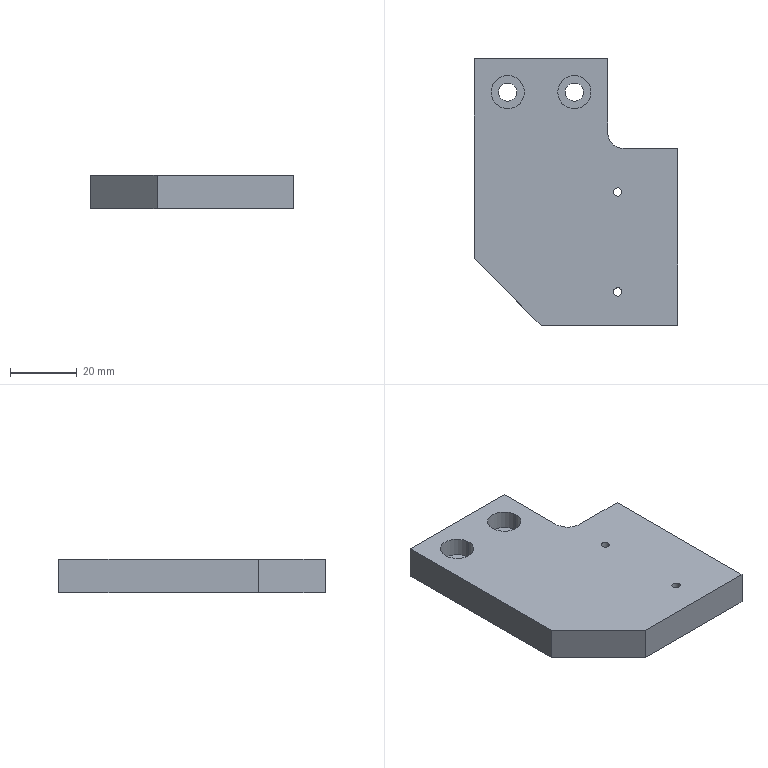Part | STEP file | PN_0025 Mount electronic clip cylinder mounting plate 4 | 1 solid | 24 faces | box 61 x 80 x 10 mm | volume 39986 mm3 | cylinder 13 | plane 11 | commonest cylinder face diameters 10 x5 2.5 x4 5.5 x4